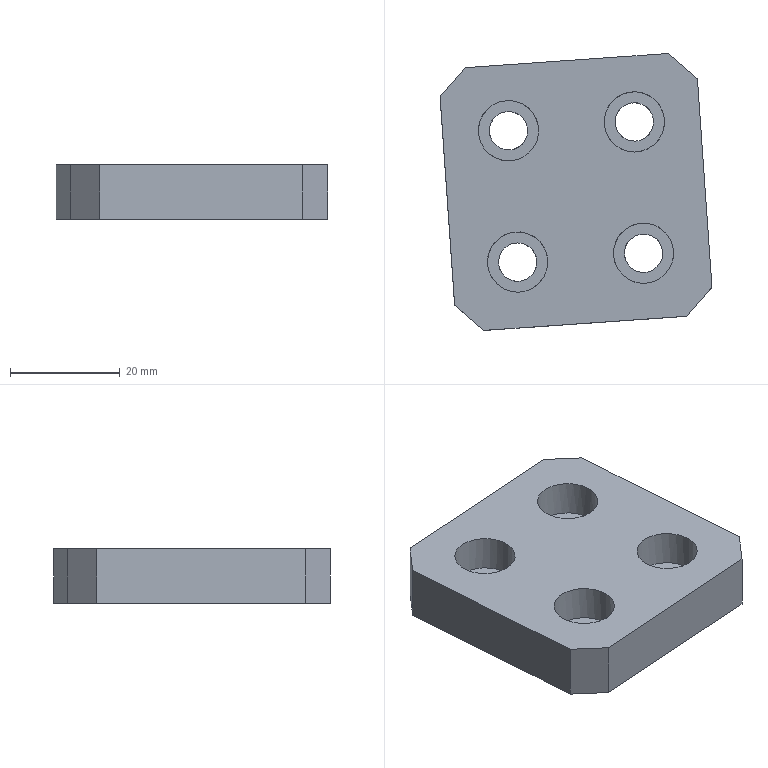Part | STEP file | 车灯-后视镜_id6_x_t | 1 solid | 22 faces | box 49.536 x 50.464 x 10 mm | volume 19050 mm3 | plane 14 | cylinder 8 | commonest cylinder face diameters 7 x4 11 x4
STEP:
#1=CARTESIAN_POINT('',(-17.5,-59.349,-255.5));
#2=VERTEX_POINT('',#1);
#3=CARTESIAN_POINT('',(19.41,-56.768,-255.5));
#4=VERTEX_POINT('',#3);
#5=CARTESIAN_POINT('',(1.531,-58.018,-255.5));
#6=DIRECTION('',(0.9976,0.06976,0.));
#7=VECTOR('',#6,1.);
#8=LINE('',#5,#7);
#9=EDGE_CURVE('',#2,#4,#8,.T.);
#10=ORIENTED_EDGE('',*,*,#9,.F.);
#11=CARTESIAN_POINT('',(-22.139,-64.685,-255.5));
#12=VERTEX_POINT('',#11);
#13=CARTESIAN_POINT('',(-27.676,-71.054,-255.5));
#14=DIRECTION('',(-0.6561,-0.7547,0.));
#15=VECTOR('',#14,1.);
#16=LINE('',#13,#15);
#17=EDGE_CURVE('',#2,#12,#16,.T.);
#18=ORIENTED_EDGE('',*,*,#17,.T.);
#19=CARTESIAN_POINT('',(-19.488,-102.593,-255.5));
#20=VERTEX_POINT('',#19);
#21=CARTESIAN_POINT('',(-19.627,-100.609,-255.5));
#22=DIRECTION('',(-0.06976,0.9976,0.));
#23=VECTOR('',#22,1.);
#24=LINE('',#21,#23);
#25=EDGE_CURVE('',#20,#12,#24,.T.);
#26=ORIENTED_EDGE('',*,*,#25,.F.);
#27=CARTESIAN_POINT('',(-14.152,-107.232,-255.5));
#28=VERTEX_POINT('',#27);
#29=CARTESIAN_POINT('',(-7.7,-112.84,-255.5));
#30=DIRECTION('',(0.7547,-0.6561,0.));
#31=VECTOR('',#30,1.);
#32=LINE('',#29,#31);
#33=EDGE_CURVE('',#20,#28,#32,.T.);
#34=ORIENTED_EDGE('',*,*,#33,.T.);
#35=CARTESIAN_POINT('',(22.758,-104.651,-255.5));
#36=VERTEX_POINT('',#35);
#37=CARTESIAN_POINT('',(4.879,-105.901,-255.5));
#38=DIRECTION('',(-0.9976,-0.06976,0.));
#39=VECTOR('',#38,1.);
#40=LINE('',#37,#39);
#41=EDGE_CURVE('',#36,#28,#40,.T.);
#42=ORIENTED_EDGE('',*,*,#41,.F.);
#43=CARTESIAN_POINT('',(27.397,-99.314,-255.5));
#44=VERTEX_POINT('',#43);
#45=CARTESIAN_POINT('',(17.686,-110.486,-255.5));
#46=DIRECTION('',(0.6561,0.7547,0.));
#47=VECTOR('',#46,1.);
#48=LINE('',#45,#47);
#49=EDGE_CURVE('',#36,#44,#48,.T.);
#50=ORIENTED_EDGE('',*,*,#49,.T.);
#51=CARTESIAN_POINT('',(24.747,-61.407,-255.5));
#52=VERTEX_POINT('',#51);
#53=CARTESIAN_POINT('',(27.259,-97.331,-255.5));
#54=DIRECTION('',(0.06976,-0.9976,0.));
#55=VECTOR('',#54,1.);
#56=LINE('',#53,#55);
#57=EDGE_CURVE('',#52,#44,#56,.T.);
#58=ORIENTED_EDGE('',*,*,#57,.F.);
#59=CARTESIAN_POINT('',(31.732,-67.479,-255.5));
#60=DIRECTION('',(-0.7547,0.6561,0.));
#61=VECTOR('',#60,1.);
#62=LINE('',#59,#61);
#63=EDGE_CURVE('',#52,#4,#62,.T.);
#64=ORIENTED_EDGE('',*,*,#63,.T.);
#65=EDGE_LOOP('',(#10,#18,#26,#34,#42,#50,#58,#64));
#66=FACE_BOUND('',#65,.T.);
#67=CARTESIAN_POINT('',(14.938,-98.668,-255.5));
#68=VERTEX_POINT('',#67);
#69=CARTESIAN_POINT('',(14.938,-93.168,-255.5));
#70=DIRECTION('',(0.,0.,1.));
#71=DIRECTION('',(0.,-1.,0.));
#72=AXIS2_PLACEMENT_3D('',#69,#70,#71);
#73=CIRCLE('',#72,5.5);
#74=EDGE_CURVE('',#68,#68,#73,.T.);
#75=ORIENTED_EDGE('',*,*,#74,.F.);
#76=EDGE_LOOP('',(#75));
#77=FACE_BOUND('',#76,.T.);
#78=CARTESIAN_POINT('',(13.264,-74.727,-255.5));
#79=VERTEX_POINT('',#78);
#80=CARTESIAN_POINT('',(13.264,-69.227,-255.5));
#81=DIRECTION('',(0.,0.,-1.));
#82=DIRECTION('',(0.,-1.,0.));
#83=AXIS2_PLACEMENT_3D('',#80,#81,#82);
#84=CIRCLE('',#83,5.5);
#85=EDGE_CURVE('',#79,#79,#84,.T.);
#86=ORIENTED_EDGE('',*,*,#85,.T.);
#87=EDGE_LOOP('',(#86));
#88=FACE_BOUND('',#87,.T.);
#89=CARTESIAN_POINT('',(-8.006,-100.273,-255.5));
#90=VERTEX_POINT('',#89);
#91=CARTESIAN_POINT('',(-8.006,-94.773,-255.5));
#92=DIRECTION('',(0.,0.,-1.));
#93=DIRECTION('',(0.,-1.,0.));
#94=AXIS2_PLACEMENT_3D('',#91,#92,#93);
#95=CIRCLE('',#94,5.5);
#96=EDGE_CURVE('',#90,#90,#95,.T.);
#97=ORIENTED_EDGE('',*,*,#96,.T.);
#98=EDGE_LOOP('',(#97));
#99=FACE_BOUND('',#98,.T.);
#100=CARTESIAN_POINT('',(-9.728,-65.332,-255.5));
#101=VERTEX_POINT('',#100);
#102=CARTESIAN_POINT('',(-9.68,-70.831,-255.5));
#103=DIRECTION('',(0.,0.,1.));
#104=DIRECTION('',(-0.008727,1.,0.));
#105=AXIS2_PLACEMENT_3D('',#102,#103,#104);
#106=CIRCLE('',#105,5.5);
#107=EDGE_CURVE('',#101,#101,#106,.T.);
#108=ORIENTED_EDGE('',*,*,#107,.F.);
#109=EDGE_LOOP('',(#108));
#110=FACE_BOUND('',#109,.T.);
#111=CARTESIAN_POINT('',(4.392,-98.93,-255.5));
#112=DIRECTION('',(0.,0.,1.));
#113=DIRECTION('',(-0.06976,0.9976,0.));
#114=AXIS2_PLACEMENT_3D('',#111,#112,#113);
#115=PLANE('',#114);
#116=ADVANCED_FACE('',(#66,#77,#88,#99,#110),#115,.T.);
#117=CARTESIAN_POINT('',(27.397,-99.314,-265.5));
#118=VERTEX_POINT('',#117);
#119=CARTESIAN_POINT('',(24.747,-61.407,-265.5));
#120=VERTEX_POINT('',#119);
#121=CARTESIAN_POINT('',(27.259,-97.331,-265.5));
#122=DIRECTION('',(-0.06976,0.9976,0.));
#123=VECTOR('',#122,1.);
#124=LINE('',#121,#123);
#125=EDGE_CURVE('',#118,#120,#124,.T.);
#126=ORIENTED_EDGE('',*,*,#125,.T.);
#127=CARTESIAN_POINT('',(24.747,-61.407,-267.5));
#128=DIRECTION('',(0.,0.,1.));
#129=VECTOR('',#128,1.);
#130=LINE('',#127,#129);
#131=EDGE_CURVE('',#120,#52,#130,.T.);
#132=ORIENTED_EDGE('',*,*,#131,.T.);
#133=ORIENTED_EDGE('',*,*,#57,.T.);
#134=CARTESIAN_POINT('',(27.397,-99.314,-267.5));
#135=DIRECTION('',(0.,0.,-1.));
#136=VECTOR('',#135,1.);
#137=LINE('',#134,#136);
#138=EDGE_CURVE('',#44,#118,#137,.T.);
#139=ORIENTED_EDGE('',*,*,#138,.T.);
#140=EDGE_LOOP('',(#126,#132,#133,#139));
#141=FACE_OUTER_BOUND('',#140,.T.);
#142=CARTESIAN_POINT('',(27.259,-97.331,-267.5));
#143=DIRECTION('',(0.9976,0.06976,0.));
#144=DIRECTION('',(0.,0.,-1.));
#145=AXIS2_PLACEMENT_3D('',#142,#143,#144);
#146=PLANE('',#145);
#147=ADVANCED_FACE('',(#141),#146,.T.);
#148=ORIENTED_EDGE('',*,*,#25,.T.);
#149=CARTESIAN_POINT('',(-22.139,-64.685,-265.5));
#150=VERTEX_POINT('',#149);
#151=CARTESIAN_POINT('',(-22.139,-64.685,-267.5));
#152=DIRECTION('',(0.,0.,-1.));
#153=VECTOR('',#152,1.);
#154=LINE('',#151,#153);
#155=EDGE_CURVE('',#12,#150,#154,.T.);
#156=ORIENTED_EDGE('',*,*,#155,.T.);
#157=CARTESIAN_POINT('',(-19.488,-102.593,-265.5));
#158=VERTEX_POINT('',#157);
#159=CARTESIAN_POINT('',(-19.627,-100.609,-265.5));
#160=DIRECTION('',(0.06976,-0.9976,0.));
#161=VECTOR('',#160,1.);
#162=LINE('',#159,#161);
#163=EDGE_CURVE('',#150,#158,#162,.T.);
#164=ORIENTED_EDGE('',*,*,#163,.T.);
#165=CARTESIAN_POINT('',(-19.488,-102.593,-267.5));
#166=DIRECTION('',(0.,0.,1.));
#167=VECTOR('',#166,1.);
#168=LINE('',#165,#167);
#169=EDGE_CURVE('',#158,#20,#168,.T.);
#170=ORIENTED_EDGE('',*,*,#169,.T.);
#171=EDGE_LOOP('',(#148,#156,#164,#170));
#172=FACE_OUTER_BOUND('',#171,.T.);
#173=CARTESIAN_POINT('',(-19.627,-100.609,-267.5));
#174=DIRECTION('',(-0.9976,-0.06976,0.));
#175=DIRECTION('',(0.,0.,1.));
#176=AXIS2_PLACEMENT_3D('',#173,#174,#175);
#177=PLANE('',#176);
#178=ADVANCED_FACE('',(#172),#177,.T.);
#179=ORIENTED_EDGE('',*,*,#163,.F.);
#180=CARTESIAN_POINT('',(-17.5,-59.349,-265.5));
#181=VERTEX_POINT('',#180);
#182=CARTESIAN_POINT('',(-27.676,-71.054,-265.5));
#183=DIRECTION('',(0.6561,0.7547,0.));
#184=VECTOR('',#183,1.);
#185=LINE('',#182,#184);
#186=EDGE_CURVE('',#150,#181,#185,.T.);
#187=ORIENTED_EDGE('',*,*,#186,.T.);
#188=CARTESIAN_POINT('',(19.41,-56.768,-265.5));
#189=VERTEX_POINT('',#188);
#190=CARTESIAN_POINT('',(1.531,-58.018,-265.5));
#191=DIRECTION('',(-0.9976,-0.06976,0.));
#192=VECTOR('',#191,1.);
#193=LINE('',#190,#192);
#194=EDGE_CURVE('',#189,#181,#193,.T.);
#195=ORIENTED_EDGE('',*,*,#194,.F.);
#196=CARTESIAN_POINT('',(31.732,-67.479,-265.5));
#197=DIRECTION('',(0.7547,-0.6561,0.));
#198=VECTOR('',#197,1.);
#199=LINE('',#196,#198);
#200=EDGE_CURVE('',#189,#120,#199,.T.);
#201=ORIENTED_EDGE('',*,*,#200,.T.);
#202=ORIENTED_EDGE('',*,*,#125,.F.);
#203=CARTESIAN_POINT('',(22.758,-104.651,-265.5));
#204=VERTEX_POINT('',#203);
#205=CARTESIAN_POINT('',(17.686,-110.486,-265.5));
#206=DIRECTION('',(-0.6561,-0.7547,0.));
#207=VECTOR('',#206,1.);
#208=LINE('',#205,#207);
#209=EDGE_CURVE('',#118,#204,#208,.T.);
#210=ORIENTED_EDGE('',*,*,#209,.T.);
#211=CARTESIAN_POINT('',(-14.152,-107.232,-265.5));
#212=VERTEX_POINT('',#211);
#213=CARTESIAN_POINT('',(4.879,-105.901,-265.5));
#214=DIRECTION('',(0.9976,0.06976,0.));
#215=VECTOR('',#214,1.);
#216=LINE('',#213,#215);
#217=EDGE_CURVE('',#212,#204,#216,.T.);
#218=ORIENTED_EDGE('',*,*,#217,.F.);
#219=CARTESIAN_POINT('',(-7.7,-112.84,-265.5));
#220=DIRECTION('',(-0.7547,0.6561,0.));
#221=VECTOR('',#220,1.);
#222=LINE('',#219,#221);
#223=EDGE_CURVE('',#212,#158,#222,.T.);
#224=ORIENTED_EDGE('',*,*,#223,.T.);
#225=EDGE_LOOP('',(#179,#187,#195,#201,#202,#210,#218,#224));
#226=FACE_BOUND('',#225,.T.);
#227=CARTESIAN_POINT('',(14.938,-89.668,-265.5));
#228=VERTEX_POINT('',#227);
#229=CARTESIAN_POINT('',(14.938,-93.168,-265.5));
#230=DIRECTION('',(0.,0.,-1.));
#231=DIRECTION('',(0.,1.,0.));
#232=AXIS2_PLACEMENT_3D('',#229,#230,#231);
#233=CIRCLE('',#232,3.5);
#234=EDGE_CURVE('',#228,#228,#233,.T.);
#235=ORIENTED_EDGE('',*,*,#234,.F.);
#236=EDGE_LOOP('',(#235));
#237=FACE_BOUND('',#236,.T.);
#238=CARTESIAN_POINT('',(13.264,-65.727,-265.5));
#239=VERTEX_POINT('',#238);
#240=CARTESIAN_POINT('',(13.264,-69.227,-265.5));
#241=DIRECTION('',(0.,0.,1.));
#242=DIRECTION('',(0.,1.,0.));
#243=AXIS2_PLACEMENT_3D('',#240,#241,#242);
#244=CIRCLE('',#243,3.5);
#245=EDGE_CURVE('',#239,#239,#244,.T.);
#246=ORIENTED_EDGE('',*,*,#245,.T.);
#247=EDGE_LOOP('',(#246));
#248=FACE_BOUND('',#247,.T.);
#249=CARTESIAN_POINT('',(-8.006,-91.273,-265.5));
#250=VERTEX_POINT('',#249);
#251=CARTESIAN_POINT('',(-8.006,-94.773,-265.5));
#252=DIRECTION('',(0.,0.,1.));
#253=DIRECTION('',(0.,1.,0.));
#254=AXIS2_PLACEMENT_3D('',#251,#252,#253);
#255=CIRCLE('',#254,3.5);
#256=EDGE_CURVE('',#250,#250,#255,.T.);
#257=ORIENTED_EDGE('',*,*,#256,.T.);
#258=EDGE_LOOP('',(#257));
#259=FACE_BOUND('',#258,.T.);
#260=CARTESIAN_POINT('',(-9.649,-74.331,-265.5));
#261=VERTEX_POINT('',#260);
#262=CARTESIAN_POINT('',(-9.68,-70.831,-265.5));
#263=DIRECTION('',(0.,0.,-1.));
#264=DIRECTION('',(0.008727,-1.,0.));
#265=AXIS2_PLACEMENT_3D('',#262,#263,#264);
#266=CIRCLE('',#265,3.5);
#267=EDGE_CURVE('',#261,#261,#266,.T.);
#268=ORIENTED_EDGE('',*,*,#267,.F.);
#269=EDGE_LOOP('',(#268));
#270=FACE_BOUND('',#269,.T.);
#271=CARTESIAN_POINT('',(4.392,-98.93,-265.5));
#272=DIRECTION('',(0.,0.,-1.));
#273=DIRECTION('',(0.06976,-0.9976,0.));
#274=AXIS2_PLACEMENT_3D('',#271,#272,#273);
#275=PLANE('',#274);
#276=ADVANCED_FACE('',(#226,#237,#248,#259,#270),#275,.T.);
#277=ORIENTED_EDGE('',*,*,#194,.T.);
#278=CARTESIAN_POINT('',(-17.5,-59.349,-267.5));
#279=DIRECTION('',(0.,0.,1.));
#280=VECTOR('',#279,1.);
#281=LINE('',#278,#280);
#282=EDGE_CURVE('',#181,#2,#281,.T.);
#283=ORIENTED_EDGE('',*,*,#282,.T.);
#284=ORIENTED_EDGE('',*,*,#9,.T.);
#285=CARTESIAN_POINT('',(19.41,-56.768,-267.5));
#286=DIRECTION('',(0.,0.,-1.));
#287=VECTOR('',#286,1.);
#288=LINE('',#285,#287);
#289=EDGE_CURVE('',#4,#189,#288,.T.);
#290=ORIENTED_EDGE('',*,*,#289,.T.);
#291=EDGE_LOOP('',(#277,#283,#284,#290));
#292=FACE_OUTER_BOUND('',#291,.T.);
#293=CARTESIAN_POINT('',(1.531,-58.018,-267.5));
#294=DIRECTION('',(-0.06976,0.9976,0.));
#295=DIRECTION('',(0.,0.,-1.));
#296=AXIS2_PLACEMENT_3D('',#293,#294,#295);
#297=PLANE('',#296);
#298=ADVANCED_FACE('',(#292),#297,.T.);
#299=CARTESIAN_POINT('',(-9.436,-74.323,-262.));
#300=VERTEX_POINT('',#299);
#301=CARTESIAN_POINT('',(-9.68,-70.831,-262.));
#302=DIRECTION('',(0.,0.,-1.));
#303=DIRECTION('',(0.06976,-0.9976,0.));
#304=AXIS2_PLACEMENT_3D('',#301,#302,#303);
#305=CIRCLE('',#304,3.5);
#306=EDGE_CURVE('',#300,#300,#305,.T.);
#307=ORIENTED_EDGE('',*,*,#306,.F.);
#308=EDGE_LOOP('',(#307));
#309=FACE_BOUND('',#308,.T.);
#310=ORIENTED_EDGE('',*,*,#267,.T.);
#311=EDGE_LOOP('',(#310));
#312=FACE_BOUND('',#311,.T.);
#313=CARTESIAN_POINT('',(-9.68,-70.831,-265.5));
#314=DIRECTION('',(0.,0.,1.));
#315=DIRECTION('',(0.06976,-0.9976,0.));
#316=AXIS2_PLACEMENT_3D('',#313,#314,#315);
#317=CYLINDRICAL_SURFACE('',#316,3.5);
#318=ADVANCED_FACE('',(#309,#312),#317,.F.);
#319=ORIENTED_EDGE('',*,*,#306,.T.);
#320=EDGE_LOOP('',(#319));
#321=FACE_BOUND('',#320,.T.);
#322=CARTESIAN_POINT('',(-9.296,-76.318,-262.));
#323=VERTEX_POINT('',#322);
#324=CARTESIAN_POINT('',(-9.68,-70.831,-262.));
#325=DIRECTION('',(0.,0.,-1.));
#326=DIRECTION('',(0.06976,-0.9976,0.));
#327=AXIS2_PLACEMENT_3D('',#324,#325,#326);
#328=CIRCLE('',#327,5.5);
#329=EDGE_CURVE('',#323,#323,#328,.T.);
#330=ORIENTED_EDGE('',*,*,#329,.F.);
#331=EDGE_LOOP('',(#330));
#332=FACE_BOUND('',#331,.T.);
#333=CARTESIAN_POINT('',(-9.68,-70.831,-262.));
#334=DIRECTION('',(0.,0.,-1.));
#335=DIRECTION('',(-0.06976,0.9976,0.));
#336=AXIS2_PLACEMENT_3D('',#333,#334,#335);
#337=PLANE('',#336);
#338=ADVANCED_FACE('',(#321,#332),#337,.F.);
#339=ORIENTED_EDGE('',*,*,#329,.T.);
#340=EDGE_LOOP('',(#339));
#341=FACE_BOUND('',#340,.T.);
#342=ORIENTED_EDGE('',*,*,#107,.T.);
#343=EDGE_LOOP('',(#342));
#344=FACE_BOUND('',#343,.T.);
#345=CARTESIAN_POINT('',(-9.68,-70.831,-255.5));
#346=DIRECTION('',(0.,0.,-1.));
#347=DIRECTION('',(-0.06976,0.9976,0.));
#348=AXIS2_PLACEMENT_3D('',#345,#346,#347);
#349=CYLINDRICAL_SURFACE('',#348,5.5);
#350=ADVANCED_FACE('',(#341,#344),#349,.F.);
#351=CARTESIAN_POINT('',(-7.762,-98.264,-262.));
#352=VERTEX_POINT('',#351);
#353=CARTESIAN_POINT('',(-8.006,-94.773,-262.));
#354=DIRECTION('',(0.,0.,1.));
#355=DIRECTION('',(0.06976,-0.9976,0.));
#356=AXIS2_PLACEMENT_3D('',#353,#354,#355);
#357=CIRCLE('',#356,3.5);
#358=EDGE_CURVE('',#352,#352,#357,.T.);
#359=ORIENTED_EDGE('',*,*,#358,.T.);
#360=EDGE_LOOP('',(#359));
#361=FACE_BOUND('',#360,.T.);
#362=ORIENTED_EDGE('',*,*,#256,.F.);
#363=EDGE_LOOP('',(#362));
#364=FACE_BOUND('',#363,.T.);
#365=CARTESIAN_POINT('',(-8.006,-94.773,-265.5));
#366=DIRECTION('',(0.,0.,1.));
#367=DIRECTION('',(-0.06976,0.9976,0.));
#368=AXIS2_PLACEMENT_3D('',#365,#366,#367);
#369=CYLINDRICAL_SURFACE('',#368,3.5);
#370=ADVANCED_FACE('',(#361,#364),#369,.F.);
#371=ORIENTED_EDGE('',*,*,#358,.F.);
#372=EDGE_LOOP('',(#371));
#373=FACE_BOUND('',#372,.T.);
#374=CARTESIAN_POINT('',(-7.622,-100.259,-262.));
#375=VERTEX_POINT('',#374);
#376=CARTESIAN_POINT('',(-8.006,-94.773,-262.));
#377=DIRECTION('',(0.,0.,1.));
#378=DIRECTION('',(0.06976,-0.9976,0.));
#379=AXIS2_PLACEMENT_3D('',#376,#377,#378);
#380=CIRCLE('',#379,5.5);
#381=EDGE_CURVE('',#375,#375,#380,.T.);
#382=ORIENTED_EDGE('',*,*,#381,.T.);
#383=EDGE_LOOP('',(#382));
#384=FACE_BOUND('',#383,.T.);
#385=CARTESIAN_POINT('',(-8.006,-94.773,-262.));
#386=DIRECTION('',(0.,0.,-1.));
#387=DIRECTION('',(0.06976,-0.9976,0.));
#388=AXIS2_PLACEMENT_3D('',#385,#386,#387);
#389=PLANE('',#388);
#390=ADVANCED_FACE('',(#373,#384),#389,.F.);
#391=ORIENTED_EDGE('',*,*,#381,.F.);
#392=EDGE_LOOP('',(#391));
#393=FACE_BOUND('',#392,.T.);
#394=ORIENTED_EDGE('',*,*,#96,.F.);
#395=EDGE_LOOP('',(#394));
#396=FACE_BOUND('',#395,.T.);
#397=CARTESIAN_POINT('',(-8.006,-94.773,-255.5));
#398=DIRECTION('',(0.,0.,-1.));
#399=DIRECTION('',(0.06976,-0.9976,0.));
#400=AXIS2_PLACEMENT_3D('',#397,#398,#399);
#401=CYLINDRICAL_SURFACE('',#400,5.5);
#402=ADVANCED_FACE('',(#393,#396),#401,.F.);
#403=CARTESIAN_POINT('',(13.508,-72.718,-262.));
#404=VERTEX_POINT('',#403);
#405=CARTESIAN_POINT('',(13.264,-69.227,-262.));
#406=DIRECTION('',(0.,0.,1.));
#407=DIRECTION('',(0.06976,-0.9976,0.));
#408=AXIS2_PLACEMENT_3D('',#405,#406,#407);
#409=CIRCLE('',#408,3.5);
#410=EDGE_CURVE('',#404,#404,#409,.T.);
#411=ORIENTED_EDGE('',*,*,#410,.T.);
#412=EDGE_LOOP('',(#411));
#413=FACE_BOUND('',#412,.T.);
#414=ORIENTED_EDGE('',*,*,#245,.F.);
#415=EDGE_LOOP('',(#414));
#416=FACE_BOUND('',#415,.T.);
#417=CARTESIAN_POINT('',(13.264,-69.227,-265.5));
#418=DIRECTION('',(0.,0.,1.));
#419=DIRECTION('',(0.06976,-0.9976,0.));
#420=AXIS2_PLACEMENT_3D('',#417,#418,#419);
#421=CYLINDRICAL_SURFACE('',#420,3.5);
#422=ADVANCED_FACE('',(#413,#416),#421,.F.);
#423=ORIENTED_EDGE('',*,*,#410,.F.);
#424=EDGE_LOOP('',(#423));
#425=FACE_BOUND('',#424,.T.);
#426=CARTESIAN_POINT('',(13.648,-74.714,-262.));
#427=VERTEX_POINT('',#426);
#428=CARTESIAN_POINT('',(13.264,-69.227,-262.));
#429=DIRECTION('',(0.,0.,1.));
#430=DIRECTION('',(0.06976,-0.9976,0.));
#431=AXIS2_PLACEMENT_3D('',#428,#429,#430);
#432=CIRCLE('',#431,5.5);
#433=EDGE_CURVE('',#427,#427,#432,.T.);
#434=ORIENTED_EDGE('',*,*,#433,.T.);
#435=EDGE_LOOP('',(#434));
#436=FACE_BOUND('',#435,.T.);
#437=CARTESIAN_POINT('',(13.264,-69.227,-262.));
#438=DIRECTION('',(0.,0.,-1.));
#439=DIRECTION('',(-0.06976,0.9976,0.));
#440=AXIS2_PLACEMENT_3D('',#437,#438,#439);
#441=PLANE('',#440);
#442=ADVANCED_FACE('',(#425,#436),#441,.F.);
#443=ORIENTED_EDGE('',*,*,#433,.F.);
#444=EDGE_LOOP('',(#443));
#445=FACE_BOUND('',#444,.T.);
#446=ORIENTED_EDGE('',*,*,#85,.F.);
#447=EDGE_LOOP('',(#446));
#448=FACE_BOUND('',#447,.T.);
#449=CARTESIAN_POINT('',(13.264,-69.227,-255.5));
#450=DIRECTION('',(0.,0.,-1.));
#451=DIRECTION('',(-0.06976,0.9976,0.));
#452=AXIS2_PLACEMENT_3D('',#449,#450,#451);
#453=CYLINDRICAL_SURFACE('',#452,5.5);
#454=ADVANCED_FACE('',(#445,#448),#453,.F.);
#455=CARTESIAN_POINT('',(15.182,-96.66,-262.));
#456=VERTEX_POINT('',#455);
#457=CARTESIAN_POINT('',(14.938,-93.168,-262.));
#458=DIRECTION('',(0.,0.,-1.));
#459=DIRECTION('',(0.06976,-0.9976,0.));
#460=AXIS2_PLACEMENT_3D('',#457,#458,#459);
#461=CIRCLE('',#460,3.5);
#462=EDGE_CURVE('',#456,#456,#461,.T.);
#463=ORIENTED_EDGE('',*,*,#462,.F.);
#464=EDGE_LOOP('',(#463));
#465=FACE_BOUND('',#464,.T.);
#466=ORIENTED_EDGE('',*,*,#234,.T.);
#467=EDGE_LOOP('',(#466));
#468=FACE_BOUND('',#467,.T.);
#469=CARTESIAN_POINT('',(14.938,-93.168,-265.5));
#470=DIRECTION('',(0.,0.,1.));
#471=DIRECTION('',(-0.06976,0.9976,0.));
#472=AXIS2_PLACEMENT_3D('',#469,#470,#471);
#473=CYLINDRICAL_SURFACE('',#472,3.5);
#474=ADVANCED_FACE('',(#465,#468),#473,.F.);
#475=ORIENTED_EDGE('',*,*,#462,.T.);
#476=EDGE_LOOP('',(#475));
#477=FACE_BOUND('',#476,.T.);
#478=CARTESIAN_POINT('',(15.322,-98.655,-262.));
#479=VERTEX_POINT('',#478);
#480=CARTESIAN_POINT('',(14.938,-93.168,-262.));
#481=DIRECTION('',(0.,0.,-1.));
#482=DIRECTION('',(0.06976,-0.9976,0.));
#483=AXIS2_PLACEMENT_3D('',#480,#481,#482);
#484=CIRCLE('',#483,5.5);
#485=EDGE_CURVE('',#479,#479,#484,.T.);
#486=ORIENTED_EDGE('',*,*,#485,.F.);
#487=EDGE_LOOP('',(#486));
#488=FACE_BOUND('',#487,.T.);
#489=CARTESIAN_POINT('',(14.938,-93.168,-262.));
#490=DIRECTION('',(0.,0.,-1.));
#491=DIRECTION('',(0.06976,-0.9976,0.));
#492=AXIS2_PLACEMENT_3D('',#489,#490,#491);
#493=PLANE('',#492);
#494=ADVANCED_FACE('',(#477,#488),#493,.F.);
#495=ORIENTED_EDGE('',*,*,#485,.T.);
#496=EDGE_LOOP('',(#495));
#497=FACE_BOUND('',#496,.T.);
#498=ORIENTED_EDGE('',*,*,#74,.T.);
#499=EDGE_LOOP('',(#498));
#500=FACE_BOUND('',#499,.T.);
#501=CARTESIAN_POINT('',(14.938,-93.168,-255.5));
#502=DIRECTION('',(0.,0.,-1.));
#503=DIRECTION('',(0.06976,-0.9976,0.));
#504=AXIS2_PLACEMENT_3D('',#501,#502,#503);
#505=CYLINDRICAL_SURFACE('',#504,5.5);
#506=ADVANCED_FACE('',(#497,#500),#505,.F.);
#507=ORIENTED_EDGE('',*,*,#217,.T.);
#508=CARTESIAN_POINT('',(22.758,-104.651,-261.5));
#509=DIRECTION('',(0.,0.,1.));
#510=VECTOR('',#509,1.);
#511=LINE('',#508,#510);
#512=EDGE_CURVE('',#204,#36,#511,.T.);
#513=ORIENTED_EDGE('',*,*,#512,.T.);
#514=ORIENTED_EDGE('',*,*,#41,.T.);
#515=CARTESIAN_POINT('',(-14.152,-107.232,-261.5));
#516=DIRECTION('',(0.,0.,-1.));
#517=VECTOR('',#516,1.);
#518=LINE('',#515,#517);
#519=EDGE_CURVE('',#28,#212,#518,.T.);
#520=ORIENTED_EDGE('',*,*,#519,.T.);
#521=EDGE_LOOP('',(#507,#513,#514,#520));
#522=FACE_OUTER_BOUND('',#521,.T.);
#523=CARTESIAN_POINT('',(4.879,-105.901,-261.5));
#524=DIRECTION('',(-0.06976,0.9976,0.));
#525=DIRECTION('',(0.,0.,1.));
#526=AXIS2_PLACEMENT_3D('',#523,#524,#525);
#527=PLANE('',#526);
#528=ADVANCED_FACE('',(#522),#527,.F.);
#529=ORIENTED_EDGE('',*,*,#209,.F.);
#530=ORIENTED_EDGE('',*,*,#138,.F.);
#531=ORIENTED_EDGE('',*,*,#49,.F.);
#532=ORIENTED_EDGE('',*,*,#512,.F.);
#533=EDGE_LOOP('',(#529,#530,#531,#532));
#534=FACE_OUTER_BOUND('',#533,.T.);
#535=CARTESIAN_POINT('',(22.758,-104.651,-261.5));
#536=DIRECTION('',(0.7547,-0.6561,0.));
#537=DIRECTION('',(0.6561,0.7547,0.));
#538=AXIS2_PLACEMENT_3D('',#535,#536,#537);
#539=PLANE('',#538);
#540=ADVANCED_FACE('',(#534),#539,.T.);
#541=ORIENTED_EDGE('',*,*,#33,.F.);
#542=ORIENTED_EDGE('',*,*,#169,.F.);
#543=ORIENTED_EDGE('',*,*,#223,.F.);
#544=ORIENTED_EDGE('',*,*,#519,.F.);
#545=EDGE_LOOP('',(#541,#542,#543,#544));
#546=FACE_OUTER_BOUND('',#545,.T.);
#547=CARTESIAN_POINT('',(-14.152,-107.232,-261.5));
#548=DIRECTION('',(-0.6561,-0.7547,0.));
#549=DIRECTION('',(0.7547,-0.6561,0.));
#550=AXIS2_PLACEMENT_3D('',#547,#548,#549);
#551=PLANE('',#550);
#552=ADVANCED_FACE('',(#546),#551,.T.);
#553=ORIENTED_EDGE('',*,*,#17,.F.);
#554=ORIENTED_EDGE('',*,*,#282,.F.);
#555=ORIENTED_EDGE('',*,*,#186,.F.);
#556=ORIENTED_EDGE('',*,*,#155,.F.);
#557=EDGE_LOOP('',(#553,#554,#555,#556));
#558=FACE_OUTER_BOUND('',#557,.T.);
#559=CARTESIAN_POINT('',(-22.139,-64.685,-267.5));
#560=DIRECTION('',(0.7547,-0.6561,0.));
#561=DIRECTION('',(0.6561,0.7547,0.));
#562=AXIS2_PLACEMENT_3D('',#559,#560,#561);
#563=PLANE('',#562);
#564=ADVANCED_FACE('',(#558),#563,.F.);
#565=ORIENTED_EDGE('',*,*,#63,.F.);
#566=ORIENTED_EDGE('',*,*,#131,.F.);
#567=ORIENTED_EDGE('',*,*,#200,.F.);
#568=ORIENTED_EDGE('',*,*,#289,.F.);
#569=EDGE_LOOP('',(#565,#566,#567,#568));
#570=FACE_OUTER_BOUND('',#569,.T.);
#571=CARTESIAN_POINT('',(19.41,-56.768,-267.5));
#572=DIRECTION('',(-0.6561,-0.7547,0.));
#573=DIRECTION('',(0.7547,-0.6561,0.));
#574=AXIS2_PLACEMENT_3D('',#571,#572,#573);
#575=PLANE('',#574);
#576=ADVANCED_FACE('',(#570),#575,.F.);
#577=CLOSED_SHELL('',(#116,#147,#178,#276,#298,#318,#338,#350,#370,#390,#402,#422,#442,#454,#474,#494,#506,#528,#540,#552,#564,#576));
#578=MANIFOLD_SOLID_BREP('',#577);
#579=(LENGTH_UNIT()NAMED_UNIT(*)SI_UNIT(.MILLI.,.METRE.));
#580=UNCERTAINTY_MEASURE_WITH_UNIT(LENGTH_MEASURE(0.00002),#579,'','');
#581=(NAMED_UNIT(*)PLANE_ANGLE_UNIT()SI_UNIT($,.RADIAN.));
#582=PLANE_ANGLE_MEASURE_WITH_UNIT(PLANE_ANGLE_MEASURE(0.01745),#581);
#583=DIMENSIONAL_EXPONENTS(0.,0.,0.,0.,0.,0.,0.);
#584=(CONVERSION_BASED_UNIT('DEGREE',#582)NAMED_UNIT(#583)PLANE_ANGLE_UNIT());
#585=(NAMED_UNIT(*)SI_UNIT($,.STERADIAN.)SOLID_ANGLE_UNIT());
#586=(GEOMETRIC_REPRESENTATION_CONTEXT(3)GLOBAL_UNCERTAINTY_ASSIGNED_CONTEXT((#580))GLOBAL_UNIT_ASSIGNED_CONTEXT((#579,#584,#585))REPRESENTATION_CONTEXT('',''));
#587=ADVANCED_BREP_SHAPE_REPRESENTATION('',(#578),#586);